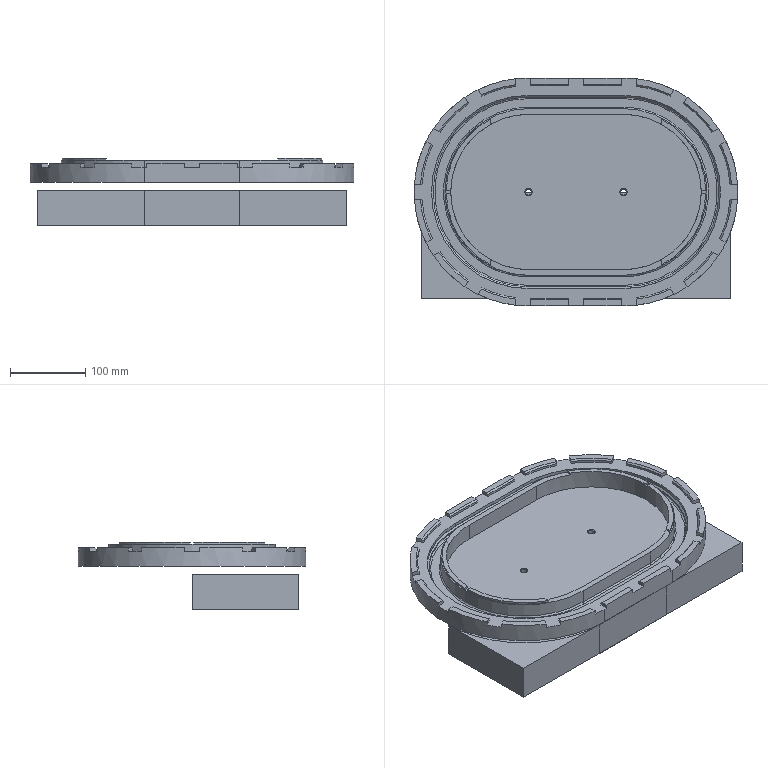NC program | NX | posted with a generic post | part box 429 x 302 x 89.371 mm
Lines 1 to 770 of 53366:
(FIXTURE OFFSET VALUES ARE NOT UNIQUE FOR OPERATION FLOOR_FACING  -- PLEASE FIX)
N10 G17 G21 G94 G90
(ADAPTIVE_MILLING , TOOL : D16开粗)
N12 T02 M6
N14 G53
N16 G17 G0 G90 X-232.529 Y-1.415 S6500 M3
N18 G43 Z20. H2
N20 Z-31.
N22 G94 G1 X-232.379 Y-1.406 Z-31.937 F3000.
N24 X-232.23 Y-1.398 Z-32.308
N26 X-232.08 Y-1.389 Z-32.58
N28 X-231.93 Y-1.381 Z-32.8
N30 X-231.78 Y-1.372 Z-32.984
N32 X-231.631 Y-1.364 Z-33.142
N34 X-231.481 Y-1.355 Z-33.28
N36 X-231.331 Y-1.347 Z-33.4
N38 X-231.181 Y-1.338 Z-33.505
N40 X-231.032 Y-1.33 Z-33.598
N42 X-230.882 Y-1.321 Z-33.679
N44 X-230.732 Y-1.313 Z-33.75
N46 X-230.582 Y-1.304 Z-33.81
N48 X-230.433 Y-1.296 Z-33.862
N50 X-230.283 Y-1.287 Z-33.905
N52 X-230.133 Y-1.279 Z-33.939
N54 X-229.983 Y-1.27 Z-33.966
N56 X-229.834 Y-1.262 Z-33.985
N58 X-229.684 Y-1.253 Z-33.996
N60 X-229.534 Y-1.245 Z-34.
N62 X-226.917 Y-1.096
N64 G3 X-225.549 Y-0.177 R1.617
N66 X-224.627 Y3.205 R11.466
N68 X-224.105 Y11.109 R67.695
N70 X-224.002 Y29.525 R929.478
N72 G1 X-224.001 Y149.336
N74 G2 X-222.03 Y154.597 R8.092
N76 X-216.722 Y158.309 R13.128
N78 X-209.837 Y159.921 R26.791
N80 X-200.067 Y160.43 R100.439
N82 X-184.767 Y160.499 R886.028
N84 G1 X212.96 Y160.5
N86 G2 X218.194 Y158.455 R8.149
N88 X221.849 Y153.13 R13.214
N90 X223.433 Y146.242 R27.174
N92 X223.93 Y136.584 R101.793
N94 X223.998 Y121.509 R876.287
N96 G1 X224. Y-149.447
N98 G2 X221.953 Y-154.681 R8.155
N100 X216.79 Y-158.27 R13.129
N102 X209.801 Y-159.912 R26.786
N104 X200.368 Y-160.412 R98.806
N106 X185.181 Y-160.485 R867.12
N108 G1 X-212.947 Y-160.499
N110 G2 X-218.096 Y-158.53 R8.104
N112 X-221.786 Y-153.276 R13.109
N114 X-223.426 Y-146.287 R26.807
N116 X-223.929 Y-136.629 R100.476
N118 X-223.998 Y-121.555 R873.122
N120 G1 X-223.999 Y-6.092
N122 G2 X-223.592 Y-0.936 R45.524
N124 G3 X-223.011 Y4.707 R170.373
N126 G1 X-222.988 Y5.977
N128 G3 X-222.621 Y13.006 R221.819
N130 X-222.505 Y32.116 R969.659
N132 G1 X-222.501 Y39.761
N134 X-222.498 Y145.061
N136 G2 X-218.605 Y153.385 R11.548
N138 X-212.066 Y157.02 R17.533
N140 X-204.007 Y158.511 R37.333
N142 X-192.881 Y158.949 R147.59
N144 X-178.031 Y158.998 R940.15
N146 G1 X-77.125 Y158.999
N148 X-75.717 Y159.132
N150 X-69.613 Y159.483
N152 X-63.5 Y159.6
N154 X63.5
N156 X69.485 Y159.488
N158 G3 X77.206 Y159.103 R215.643
N160 X93.38 Y159.005 R838.433
N162 G1 X103.274 Y159.
N164 X208.573 Y158.996
N166 G2 X216.893 Y155.099 R11.533
N168 X220.497 Y148.642 R17.473
N170 X222.005 Y140.586 R36.848
N172 X222.455 Y128.786 R152.827
N174 G1 X222.498 Y115.173
N176 X222.499 Y13.629
N178 X222.631 Y12.223
N180 X222.983 Y6.118
N182 X223.1 Y0.005
N184 X222.983 Y-6.108
N186 G3 X222.61 Y-13.03 R293.259
N188 X222.504 Y-29.867 R840.804
N190 G1 X222.5 Y-37.287
N192 Y-144.836
N194 G2 X218.756 Y-153.229 R11.495
N196 X212.224 Y-156.955 R17.308
N198 X204.172 Y-158.483 R36.616
N200 X192.484 Y-158.94 R149.137
N202 X178.872 Y-158.985 R897.131
N204 G1 X77.226 Y-158.989
N206 X75.717 Y-159.132
N208 X69.613 Y-159.483
N210 X63.5 Y-159.6
N212 X-63.5
N214 X-69.485 Y-159.488
N216 G3 X-77.634 Y-159.092 R207.139
N218 X-95.274 Y-158.996 R929.441
N220 G1 X-208.336 Y-159.
N222 G2 X-216.884 Y-155.102 R11.537
N224 X-220.524 Y-148.547 R17.523
N226 X-222.012 Y-140.487 R37.347
N228 X-222.455 Y-128.798 R153.736
N230 G1 X-222.497 Y-115.186
N232 X-222.499 Y-13.648
N234 X-222.618 Y-12.392
N236 X-222.977 Y-6.275
N238 X-223.1 Y-0.15
N240 X-222.988 Y5.977
N242 X-222.641 Y12.094
N244 X-222.06 Y18.194
N246 X-221.379 Y23.365
N248 G3 X-221.041 Y33.74 R150.871
N250 G1 X-221.003 Y46.401
N252 X-221.002 Y140.561
N254 G2 X-219.826 Y146.816 R14.804
N256 X-214.016 Y153.235 R14.585
N258 X-206.467 Y156.113 R23.96
N260 X-196.979 Y157.221 R59.53
N262 X-181.908 Y157.487 R337.478
N264 G1 X-174.258 Y157.497
N266 X-89.329 Y157.498
N268 G3 X-87.862 Y157.73 R13.362
N270 G1 X-81.802 Y158.547
N272 X-76.987 Y159.01
N274 X-81.802 Y158.547
N276 X-87.862 Y157.73
N278 G2 X-92.626 Y156.952 R81.131
N280 X-100.369 Y156.639 R93.258
N282 G1 X-112.778 Y156.599
N284 X-174.266 Y156.597
N286 G3 X-193.614 Y156.428 R682.499
N288 X-203.585 Y155.591 R77.967
N290 X-210.899 Y153.436 R27.183
N292 X-217.003 Y148.242 R14.556
N294 X-219.311 Y142.035 R17.243
N296 X-219.99 Y134.422 R50.706
N298 X-220.102 Y117.548 R684.834
N300 G1 X-220.103 Y47.253
N302 G2 X-220.211 Y30.219 R872.426
N304 G1 X-221.244 Y24.267
N306 X-221.409 Y23.04
N308 X-221.244 Y24.267
N310 X-220.197 Y30.304
N312 G3 X-219.238 Y34.912 R118.578
N314 X-218.707 Y43.058 R70.838
N316 X-218.602 Y62.936 R967.012
N318 G1 X-218.601 Y119.273
N320 G2 X-218.463 Y133.672 R440.696
N322 X-217.731 Y140.6 R40.905
N324 X-210.721 Y150.549 R15.216
N326 X-203.011 Y153.582 R24.515
N328 X-193.421 Y154.775 R58.816
N330 X-178.351 Y155.082 R304.745
N332 G1 X-170.251 Y155.096
N334 X-114.418 Y155.098
N336 G3 X-100.896 Y155.158 R824.714
N338 G2 X-93.885 Y156.681 R503.045
N340 G1 X-91.557 Y157.086
N342 X-93.885 Y156.681
N344 X-99.864 Y155.402
N346 G2 X-103.132 Y154.666 R28.054
N348 X-109.994 Y154.271 R63.977
N350 X-124.591 Y154.198 R822.936
N352 G1 X-169.541 Y154.196
N354 G3 X-189.339 Y154.02 R694.539
N356 X-199.536 Y153.182 R83.166
N358 X-207.296 Y150.944 R28.996
N360 X-215.784 Y141.611 R15.806
N362 X-217.281 Y134.243 R30.094
N364 X-217.672 Y123.791 R127.733
N366 G1 X-217.702 Y110.966
N368 X-217.703 Y58.729
N370 G2 X-217.881 Y41.554 R516.659
N372 G1 X-217.963 Y40.058
N374 G3 X-219.317 Y34.426 R101.735
N376 G2 X-217.963 Y40.058 R101.735
N378 G3 X-217.086 Y43.448 R419.213
N380 X-216.413 Y49.955 R43.811
N382 X-216.207 Y64.518 R365.227
N384 G1 X-216.202 Y72.836
N386 X-216.199 Y114.524
N388 G2 X-216.023 Y129.146 R383.662
N390 X-215.134 Y136.961 R45.597
N392 X-211.69 Y144.344 R17.332
N394 X-204.611 Y149.501 R18.475
N396 X-196.373 Y151.708 R33.165
N398 X-185.273 Y152.54 R95.162
N400 X-163.562 Y152.697 R888.938
N402 G1 X-125.668 Y152.698
N404 G3 X-109.55 Y152.821 R598.221
N406 G1 X-109.313 Y152.854
N408 G2 X-101.864 Y154.893 R118.972
N410 G3 X-110.176 Y152.599 R133.755
N412 G2 X-115.078 Y151.998 R26.106
N414 X-128.084 Y151.801 R294.067
N416 G1 X-133.028 Y151.798
N418 X-165.041 Y151.796
N420 G3 X-185.177 Y151.621 R728.917
N422 X-195.823 Y150.767 R88.315
N424 X-203.814 Y148.524 R30.934
N426 X-213.134 Y138.522 R17.107
N428 X-214.778 Y130.957 R31.176
N430 X-215.254 Y120.621 R113.28
N432 X-215.301 Y106.109 R907.702
N434 G1 X-215.303 Y68.742
N436 G2 X-215.474 Y51.781 R519.848
N438 X-215.711 Y47.993 R58.537
N440 G1 X-217.207 Y42.922
N442 G2 X-214.923 Y50.388 R168.049
N444 G3 X-214.122 Y56.177 R32.13
N446 X-213.83 Y67.138 R197.125
N448 G1 X-213.802 Y80.374
N450 X-213.8 Y109.124
N452 G2 X-213.632 Y124.422 R448.239
N454 X-212.785 Y132.808 R55.119
N456 X-210.096 Y139.93 R20.672
N458 X-202.625 Y146.474 R18.231
N460 X-194.156 Y149.085 R31.148
N462 X-183.409 Y150.071 R81.805
N464 X-164.174 Y150.293 R571.096
N466 G1 X-157.311 Y150.297
N468 X-131.858 Y150.299
N470 G3 X-117.275 Y150.464 R399.813
N472 X-116.456 Y150.541 R5.706
N474 G1 X-111.653 Y152.163
N476 X-110.142 Y152.609
N478 X-111.653 Y152.163
N480 G2 X-117.413 Y150.235 R545.021
N482 X-122.514 Y149.607 R26.689
N484 X-134.835 Y149.402 R272.839
N486 G1 X-139.778 Y149.398
N488 X-160.428 Y149.396
N490 G3 X-181.127 Y149.225 R789.564
N492 X-192.114 Y148.387 R95.379
N494 X-200.459 Y146.139 R33.132
N496 X-210.577 Y135.496 R18.152
N498 X-212.338 Y127.494 R32.811
N500 X-212.843 Y117.16 R113.078
N502 X-212.902 Y100.623 R967.326
N504 G1 X-212.904 Y76.729
N506 G2 X-213.087 Y59.665 R500.906
N508 X-213.44 Y54.677 R64.548
N510 G3 X-215.012 Y50.08 R526.691
N512 G2 X-212.748 Y56.461 R110.245
N514 G3 X-211.846 Y61.666 R25.257
N516 X-211.457 Y71.559 R135.437
N518 X-211.402 Y87.236 R942.517
N520 G1 X-211.4 Y104.399
N522 G2 X-211.242 Y120.147 R508.259
N524 X-210.384 Y129.211 R62.267
N526 X-207.781 Y136.604 R22.953
N528 X-199.911 Y143.847 R18.735
N530 X-191.359 Y146.58 R31.313
N532 X-180.73 Y147.632 R78.833
N534 X-163.183 Y147.888 R458.463
N536 G1 X-152.721 Y147.897
N538 X-138.834 Y147.899
N540 G3 X-124.489 Y148.081 R360.078
N542 X-122.708 Y148.211 R16.953
N544 G2 X-117.019 Y150.351 R524.72
N546 G3 X-123.159 Y148.03 R553.774
N548 G2 X-127.343 Y147.323 R18.935
N550 X-137.456 Y147.019 R146.156
N552 G1 X-145.741 Y146.998
N554 X-156.716 Y146.996
N556 G3 X-177.302 Y146.83 R821.488
N558 X-188.517 Y146.014 R102.546
N560 X-197.208 Y143.771 R35.317
N562 X-205.569 Y137.284 R19.163
N564 X-209.058 Y129.285 R22.631
N566 X-210.227 Y120.259 R51.32
N568 X-210.493 Y105.863 R292.52
N570 G1 X-210.502 Y98.213
N572 X-210.504 Y83.817
N574 G2 X-210.697 Y66.536 R493.875
N576 X-211.165 Y60.586 R65.041
N578 X-211.536 Y59.644 R8.23
N580 G1 X-212.777 Y56.384
N582 G2 X-210.523 Y62.026 R88.882
N584 G3 X-209.526 Y67.119 R22.594
N586 X-209.067 Y77.308 R121.258
N588 X-209.004 Y90.5 R803.915
N590 G1 X-208.996 Y103.412
N592 G2 X-208.764 Y118.259 R341.857
N594 X-207.712 Y127.186 R53.849
N596 X-204.575 Y134.855 R22.208
N598 X-196.507 Y141.622 R19.769
N600 X-187.686 Y144.256 R33.605
N602 X-176.826 Y145.25 R86.624
N604 X-158.154 Y145.49 R531.312
N606 G1 X-147.27 Y145.497
N608 G3 X-131.761 Y145.647 R487.614
N610 X-128.321 Y145.871 R68.566
N612 G1 X-128.099 Y145.928
N614 X-123.159 Y148.03
N616 G2 X-128.816 Y145.645 R224.786
N618 X-132.979 Y144.939 R20.115
N620 X-143.308 Y144.62 R146.421
N622 G1 X-155.395 Y144.593
N624 G3 X-175.194 Y144.386 R644.825
N626 X-186.175 Y143.477 R93.764
N628 X-194.823 Y141.082 R34.447
N630 X-203.82 Y133.328 R19.496
N632 X-206.84 Y125.249 R25.301
N634 X-207.877 Y115.753 R61.175
N636 X-208.095 Y101.243 R367.634
N638 G1 X-208.105 Y90.005
N640 G2 X-208.295 Y72.943 R496.233
N642 X-208.899 Y65.865 R61.317
N644 X-209.138 Y65.282 R4.531
N646 G1 X-210.547 Y61.969
N648 G2 X-208.252 Y67.195 R119.991
N650 G3 X-207.2 Y72.151 R21.284
N652 X-206.692 Y81.725 R106.769
N654 X-206.599 Y98.156 R894.507
N656 G2 X-206.385 Y114.354 R417.318
N658 X-205.414 Y123.519 R61.188
N660 X-202.505 Y131.405 R24.313
N662 X-193.932 Y139.04 R20.065
N664 X-185.143 Y141.753 R33.55
N666 X-173.953 Y142.831 R84.518
N668 X-157.194 Y143.084 R458.578
N670 G1 X-145.952 Y143.111
N672 G3 X-134.898 Y143.397 R173.963
N674 X-133.171 Y143.587 R13.575
N676 X-128.474 Y145.769 R267.332
N678 G1 X-133.444 Y143.44
N680 G2 X-137.038 Y142.67 R14.728
N682 X-145.071 Y142.263 R87.833
N684 X-160.048 Y142.172 R967.726
N686 G3 X-175.904 Y141.797 R299.023
N688 X-186.271 Y140.47 R65.391
N690 X-194.54 Y137.316 R28.173
N692 X-203.021 Y127.106 R19.971
N694 X-204.989 Y118.69 R34.917
N696 X-205.61 Y108.025 R106.855
N698 X-205.711 Y91.485 R913.213
N700 G2 X-205.992 Y76.759 R299.721
N702 X-206.668 Y70.553 R45.214
N704 G1 X-208.383 Y66.884
N706 G2 X-206.008 Y71.86 R296.464
N708 G3 X-204.919 Y76.452 R19.24
N710 X-204.319 Y85.92 R89.818
N712 X-204.175 Y102.001 R941.513
N714 G2 X-203.754 Y114.816 R181.419
N716 X-202.312 Y123.342 R42.863
N718 X-197.578 Y131.934 R21.081
N720 X-189.315 Y137.394 R22.316
N722 X-179.94 Y139.69 R40.337
N724 X-167.712 Y140.532 R115.893
N726 X-150.024 Y140.714 R917.51
N728 G3 X-139.469 Y141.06 R145.435
N730 X-137.692 Y141.292 R10.352
N732 G1 X-134.315 Y143.029
N734 X-133.399 Y143.461
N736 G3 X-137.877 Y141.18 R113.782
N738 G2 X-141.24 Y140.36 R12.781
N740 X-149.269 Y139.876 R77.466
N742 X-162.445 Y139.724 R997.313
N744 G3 X-176.266 Y139.128 R177.234
N746 X-185.993 Y137.362 R49.79
N748 X-194.278 Y133.151 R24.354
N750 X-200.723 Y123.933 R20.835
N752 X-202.616 Y115.386 R37.202
N754 X-203.224 Y104.156 R118.396
N756 X-203.338 Y91.539 R848.814
N758 G2 X-203.751 Y79.751 R171.159
N760 X-204.436 Y74.878 R34.133
N762 G1 X-206.136 Y71.572
N764 X-203.715 Y76.265
N766 G3 X-202.562 Y80.981 R19.372
N768 X-201.946 Y89.782 R82.903
N770 X-201.736 Y102.722 R902.7
N772 G2 X-201.138 Y113.952 R121.489
N774 X-199.225 Y122.495 R35.576
N776 X-189.076 Y133.824 R20.616
N778 X-180.128 Y136.775 R33.287
N780 X-169.063 Y137.966 R79.662
N782 X-155.447 Y138.285 R378.224
N784 G3 X-144.611 Y138.641 R167.502
N786 X-142.021 Y138.957 R20.136
N788 G1 X-141.794 Y139.044
N790 G2 X-137.844 Y141.197 R66.863
N792 G3 X-142.088 Y138.877 R70.749
N794 G2 X-145.474 Y138.006 R12.512
N796 X-153.148 Y137.476 R71.347
N798 G1 X-164.09 Y137.234
N800 G3 X-176.317 Y136.379 R117.575
N802 X-185.689 Y134.075 R39.995
N804 X-194.12 Y128.323 R21.894
N806 X-198.764 Y119.769 R22.771
N808 X-200.389 Y110.705 R44.506
N810 X-200.873 Y99.13 R167.521
N812 G2 X-201.233 Y86.251 R299.634
N814 X-202.123 Y79.17 R45.234
N816 G1 X-202.246 Y78.819
N818 X-203.811 Y76.05
N820 X-201.482 Y80.193
N822 G3 X-200.258 Y84.8 R18.25
N824 X-199.559 Y93.549 R80.328
N826 G2 X-199.157 Y105.736 R888.13
N828 X-198.059 Y115.339 R63.526
N830 X-194.989 Y123.52 R26.02
N832 X-186.036 Y131.565 R21.185
N834 X-176.934 Y134.434 R34.78
N836 X-165.975 Y135.574 R84.23
N838 X-153.798 Y135.971 R849.201
N840 G3 X-146.27 Y136.57 R64.398
N842 X-145.763 Y136.75 R4.13
N844 G2 X-142.024 Y138.914 R85.291
N846 G3 X-146.05 Y136.572 R95.169
N848 G2 X-149.311 Y135.66 R11.602
N850 X-156.846 Y135.036 R68.442
N852 G3 X-168.491 Y134.485 R359.878
N854 X-178.721 Y132.991 R62.429
N856 X-187.217 Y129.504 R28.342
N858 X-195.619 Y119.119 R21.192
N860 X-197.729 Y110.276 R36.881
N862 X-198.455 Y99.505 R121.199
N864 G2 X-199.004 Y88.472 R198.973
N866 X-199.881 Y82.931 R35.355
N868 G1 X-199.982 Y82.695
N870 G3 X-201.63 Y79.902 R56.352
N872 G2 X-199.389 Y83.651 R71.76
N874 G3 X-198.103 Y87.599 R14.334
N876 X-197.23 Y95.299 R59.584
N878 G2 X-196.596 Y105.782 R494.055
N880 X-195.152 Y114.653 R49.361
N882 X-190.883 Y123.269 R23.267
N884 X-182.366 Y129.607 R22.421
N886 X-173.186 Y132.197 R38.111
N888 X-162.553 Y133.236 R99.8
N890 G3 X-153.14 Y133.81 R258.501
N892 X-149.863 Y134.27 R33.895
N894 G1 X-149.551 Y134.399
N896 X-146.014 Y136.594
N898 X-149.838 Y134.221
N900 G2 X-152.962 Y133.282 R11.534
N902 X-159.312 Y132.579 R62.01
N904 G3 X-169.26 Y131.76 R217.506
N906 X-178.931 Y129.727 R47.487
N908 X-187.326 Y125.027 R24.367
N910 X-193.497 Y115.66 R22.216
N912 X-195.415 Y107. R40.564
N914 X-196.199 Y97.313 R169.715
N916 G2 X-197.097 Y88.799 R77.617
N918 X-197.634 Y86.505 R18.479
N920 G1 X-199.409 Y83.618
N922 X-197.031 Y87.422
N924 G3 X-195.672 Y91.568 R15.382
N926 X-194.767 Y98.229 R66.194
N928 G2 X-193.781 Y107.15 R159.087
N930 X-191.492 Y115.603 R34.646
N932 X-181.082 Y126.549 R21.644
N934 X-171.899 Y129.546 R35.313
N936 X-162.868 Y130.732 R90.72
N938 G3 X-155.159 Y131.552 R127.176
N940 X-153.358 Y131.913 R13.814
N942 G1 X-153.124 Y132.025
N944 G2 X-149.772 Y134.261 R152.245
N946 G3 X-153.404 Y131.836 R162.206
N948 G2 X-156.364 Y130.842 R11.194
N950 X-162.337 Y129.946 R65.092
N952 G3 X-171.462 Y128.612 R104.727
N954 X-180.279 Y125.63 R34.085
N956 X-190.699 Y114.087 R21.884
N958 X-192.935 Y105.501 R38.719
N960 X-194.031 Y96.683 R281.796
N962 G2 X-195.27 Y90.134 R40.815
N964 G1 X-195.435 Y89.757
N966 X-197.197 Y87.147
N968 G3 X-194.621 Y90.996 R147.309
N970 X-193.131 Y95.401 R17.491
N972 X-191.826 Y102.887 R141.538
N974 G2 X-189.876 Y111.086 R48.243
N976 X-183.95 Y120.383 R22.723
N978 X-175.286 Y125.52 R25.341
N980 X-166.121 Y127.772 R50.643
N982 G3 X-158.637 Y128.978 R282.809
N984 X-156.942 Y129.391 R10.268
N986 G1 X-156.745 Y129.499
N988 G2 X-153.359 Y131.866 R63.417
N990 G3 X-157.017 Y129.299 R66.548
N992 G2 X-160.043 Y128.163 R11.885
N994 X-166.732 Y126.768 R133.646
N996 G3 X-175.273 Y124.351 R47.644
N998 X-183.883 Y118.583 R23.72
N1000 X-188.97 Y109.888 R24.411
N1002 X-190.989 Y101.819 R55.382
N1004 G2 X-192.449 Y94.84 R91.224
N1006 X-192.949 Y93.327 R9.609
N1008 G3 X-194.793 Y90.707 R70.089
N1010 G2 X-192.275 Y94.233 R81.048
N1012 G3 X-190.655 Y98.1 R16.248
N1014 X-188.866 Y104.735 R322.928
N1016 G2 X-185.871 Y112.374 R34.392
N1018 X-175.833 Y121.824 R23.043
N1020 X-167.581 Y124.777 R41.314
N1022 G3 X-161.416 Y126.325 R379.706
N1024 X-160.25 Y126.931 R2.341
N1026 G1 X-156.983 Y129.324
N1028 G3 X-160.86 Y126.448 R130.955
N1030 G2 X-163.791 Y125.124 R13.101
N1032 G1 X-169.878 Y123.158
N1034 G3 X-177.662 Y119.409 R32.564
N1036 X-185.861 Y109.566 R23.743
N1038 X-188.386 Y102.579 R50.642
N1040 G2 X-190.092 Y97.248 R73.13
N1042 X-190.425 Y96.758 R3.493
N1044 G1 X-192.286 Y94.217
N1046 G2 X-189.397 Y98.055 R72.895
N1048 G3 X-187.482 Y101.798 R21.048
N1050 G2 X-184.801 Y107.935 R97.855
N1052 X-176.996 Y117.321 R25.289
N1054 X-169.357 Y121.384 R35.147
N1056 G1 X-165.354 Y122.931
N1058 X-165.041 Y123.133
N1060 X-160.81 Y126.488
N1062 X-165.677 Y122.617
N1064 G2 X-168.65 Y120.939 R26.85
N1066 G3 X-174.528 Y117.682 R58.062
N1068 X-183.554 Y107.751 R27.028
N1070 X-186.48 Y101.769 R113.604
N1072 G1 X-186.626 Y101.549
N1074 X-189.422 Y98.023
N1076 G2 X-184.803 Y103.688 R132.321
N1078 G3 X-181.624 Y108.167 R498.29
N1080 G2 X-171.953 Y117.078 R33.192
N1082 G3 X-169.682 Y119.153 R55.725
N1084 G1 X-165.412 Y122.814
N1086 X-169.682 Y119.153
N1088 X-174.168 Y114.999
N1090 X-178.492 Y110.676
N1092 X-182.646 Y106.19
N1094 X-184.916 Y103.543
N1096 G2 X-186.671 Y103.077 R1.603
N1098 G1 X-189.668 Y104.035 Z-33.9
N1100 X-190.008 Y104.146 F15000.
N1102 X-190.352 Y104.242
N1104 G3 X-191.997 Y103.543 R1.6
N1106 G1 X-201.643 Y88.697
N1108 G3 X-209.964 Y74.237 R156.698
N1110 X-219.209 Y52.045 R153.871
N1112 X-222.647 Y40.259 R185.878
N1114 X-226.149 Y22.272 R159.931
N1116 X-227.008 Y14.46 R192.013
N1118 X-227.982 Y1.392 R369.431
N1120 G1 X-228.631 Y-10.074
N1122 G3 X-227.238 Y-11.752 R1.6
N1124 G1 X-226.609 Y-11.833
N1126 X-225.182 Y-12.013 Z-33.946 F3000.
N1128 X-223.755 Y-12.205 Z-33.991
N1130 X-223.499 Y-12.284 Z-34.
N1132 G2 X-222.499 Y-13.615 R1.6
N1134 X-221.814 Y-20.81 R304.339
N1136 X-221.608 Y-32.307 R229.116
N1138 G1 X-221.599 Y-41.066
N1140 X-221.597 Y-115.829
N1142 G3 X-221.431 Y-134.165 R623.958
N1144 X-220.634 Y-143.348 R69.881
N1146 X-218.547 Y-150.098 R23.675
N1148 X-211.468 Y-156.376 R12.438
N1150 X-204.764 Y-157.746 R25.7
N1152 X-195.434 Y-158.073 R120.939
N1154 G1 X-183.622 Y-158.099
N1156 X-93.994 Y-158.097
N1158 X-84.972 Y-158.122
N1160 X-81.421 Y-158.591
N1162 X-75.461 Y-159.151
N1164 X-81.421 Y-158.591
N1166 X-87.355 Y-157.807
N1168 G3 X-91.838 Y-157.065 R139.171
N1170 X-101.536 Y-156.65 R109.757
N1172 X-117.549 Y-156.597 R976.687
N1174 G1 X-187.136 Y-156.596
N1176 G2 X-200.409 Y-156.429 R328.503
N1178 X-207.1 Y-155.613 R35.748
N1180 X-215.62 Y-149.538 R13.905
N1182 X-218.598 Y-142.279 R22.394
N1184 X-219.774 Y-133.254 R53.604
N1186 X-220.083 Y-118.634 R283.141
N1188 G1 X-220.097 Y-109.297
N1190 X-220.098 Y-44.279
N1192 G3 X-220.136 Y-30.613 R896.441
N1194 G1 X-221.199 Y-24.562
N1196 X-221.988 Y-18.765
N1198 X-221.199 Y-24.562
N1200 X-220.136 Y-30.613
N1202 G2 X-219.367 Y-36.566 R28.313
N1204 X-219.205 Y-48.39 R315.265
N1206 G1 X-219.199 Y-55.803
N1208 X-219.197 Y-109.866
N1210 G3 X-219.037 Y-128.764 R695.637
N1212 X-218.22 Y-138.736 R78.589
N1214 X-216.06 Y-146.049 R26.602
N1216 X-207.799 Y-153.619 R14.776
N1218 X-200.461 Y-155.239 R28.04
N1220 X-190.461 Y-155.661 R112.868
N1222 G1 X-177.524 Y-155.699
N1224 X-114.354
N1226 G2 X-97.8 Y-155.853 R561.178
N1228 G1 X-93.256 Y-156.802
N1230 X-91.37 Y-157.123
N1232 G2 X-97.775 Y-155.856 R123.101
N1234 X-101.588 Y-154.971 R83.467
N1236 G3 X-108.769 Y-154.355 R52.906
N1238 X-125.651 Y-154.199 R560.051
N1240 G1 X-175.236
N1242 G2 X-193.21 Y-154.085 R755.921
N1244 X-201.387 Y-153.4 R58.826
N1246 X-207.646 Y-151.294 R19.204
N1248 X-213.883 Y-144.687 R16.178
N1250 X-216.447 Y-137.007 R27.162
N1252 X-217.46 Y-127.054 R69.261
N1254 X-217.69 Y-110.857 R429.837
N1256 G1 X-217.698 Y-100.057
N1258 X-217.701 Y-52.048
N1260 G3 X-217.786 Y-40.811 R697.321
N1262 X-218.85 Y-36.587 R190.96
N1264 G1 X-219.797 Y-32.188
N1266 G3 X-217.804 Y-40.675 R133.401
N1268 G2 X-217.025 Y-45.791 R22.201
N1270 X-216.809 Y-56.386 R211.425
N1272 G1 X-216.798 Y-64.466
N1274 X-216.796 Y-104.691
N1276 G3 X-216.627 Y-124.489 R715.462
N1278 X-215.784 Y-134.798 R82.881
N1280 X-213.532 Y-142.556 R28.702
N1282 X-204.379 Y-151.036 R16.337
N1284 X-196.72 Y-152.767 R29.917
N1286 X-186.61 Y-153.248 R108.619
N1288 X-171.31 Y-153.298 R931.317
N1290 G1 X-126.279
N1292 G2 X-109.317 Y-153.468 R529.07
N1294 X-106.681 Y-153.623 R35.142
N1296 G3 X-101.321 Y-155.027 R100.077
N1298 G2 X-109.491 Y-152.811 R137.348
N1300 G3 X-115.352 Y-152.077 R35.4
N1302 X-128.478 Y-151.81 R259.983
N1304 G1 X-139.261 Y-151.798
N1306 X-175.099 Y-151.796
N1308 G2 X-190.509 Y-151.614 R411.776
N1310 X-198.776 Y-150.713 R50.837
N1312 X-205.814 Y-147.843 R19.303
N1314 X-211.674 Y-140.825 R17.766
N1316 X-214.128 Y-132.771 R30.284
N1318 X-215.085 Y-122.247 R79.668
N1320 X-215.292 Y-104.924 R529.268
N1322 G1 X-215.298 Y-95.587
N1324 X-215.299 Y-63.184
N1326 G3 X-215.45 Y-48.905 R404.662
N1328 X-215.585 Y-48.396 R4.353
N1330 G2 X-217.498 Y-41.869 R232.953
N1332 G3 X-215.198 Y-49.588 R202.063
N1334 G2 X-214.606 Y-54.403 R26.507
N1336 X-214.401 Y-67.397 R283.072
N1338 G1 X-214.398 Y-72.341
N1340 X-214.396 Y-100.303
N1342 G3 X-214.233 Y-120.102 R761.481
N1344 X-213.405 Y-130.864 R91.575
N1346 X-211.179 Y-138.976 R31.496
N1348 X-201.01 Y-148.57 R17.559
N1350 X-193.126 Y-150.33 R32.018
N1352 X-183.018 Y-150.837 R109.295
N1354 X-167.718 Y-150.898 R896.73
N1356 G1 X-135.391 Y-150.899
N1358 G2 X-118.324 Y-151.077 R514.395
N1360 X-114.001 Y-151.371 R44.635
N1362 G3 X-109.485 Y-152.813 R97.147
N1364 G2 X-114.001 Y-151.371 R97.147
N1366 G3 X-117.025 Y-150.422 R38.254
N1368 X-123.315 Y-149.668 R39.048
N1370 X-138.146 Y-149.405 R320.002
N1372 G1 X-146.461 Y-149.398
N1374 X-170.261 Y-149.396
N1376 G2 X-185.897 Y-149.234 R487.426
N1378 X-194.736 Y-148.384 R60.418
N1380 X-202.107 Y-145.733 R22.141
N1382 X-209.074 Y-137.949 R18.344
N1384 X-211.661 Y-129.594 R31.14
N1386 X-212.649 Y-119.299 R78.789
N1388 X-212.888 Y-102.426 R457.064
N1390 G1 X-212.897 Y-92.976
N1392 X-212.899 Y-71.171
N1394 G3 X-213.051 Y-57.019 R411.123
N1396 X-213.157 Y-55.43 R15.354
N1398 G2 X-215.279 Y-49.298 R191.25
N1400 G1 X-213.616 Y-54.198
N1402 G2 X-212.822 Y-56.403 R20.928
N1404 X-212.212 Y-61.382 R28.002
N1406 X-212.002 Y-73.7 R267.247
N1408 G1 X-211.998 Y-78.641
N1410 X-211.996 Y-95.916
N1412 G3 X-211.827 Y-116.39 R784.557
N1414 X-210.993 Y-127.377 R96.027
N1416 X-208.722 Y-135.827 R33.431
N1418 X-197.887 Y-146.096 R18.499
N1420 X-189.782 Y-147.899 R33.534
N1422 X-178.775 Y-148.44 R116.099
N1424 X-163.475 Y-148.498 R914.647
N1426 G1 X-142.929 Y-148.5
N1428 G2 X-125.761 Y-148.694 R484.531
N1430 X-120.374 Y-149.106 R60.989
N1432 G1 X-116.358 Y-150.593
N1434 G3 X-122.503 Y-148.32 R554.363
N1436 X-128.107 Y-147.407 R27.729
N1438 X-138.422 Y-147.044 R149.956
N1440 X-153.661 Y-146.999 R963.406
N1442 G1 X-165.874 Y-146.996
N1444 G2 X-182.634 Y-146.813 R483.698
N1446 X-191.803 Y-145.885 R60.743
N1448 X-199.272 Y-143.166 R23.24
N1450 X-206.527 Y-135.116 R19.039
N1452 X-209.187 Y-126.651 R31.809
N1454 X-210.238 Y-115.911 R79.881
N1456 X-210.486 Y-99.263 R446.992
N1458 G1 X-210.496 Y-90.938
N1460 X-210.497 Y-80.393
N1462 G3 X-210.64 Y-64.42 R515.325
N1464 X-210.828 Y-61.379 R36.427
N1466 X-211.425 Y-59.921 R12.938
N1468 G1 X-212.993 Y-55.823
N1470 G3 X-210.71 Y-61.591 R113.852
N1472 G2 X-209.99 Y-65.322 R15.9
N1474 X-209.633 Y-74.656 R112.492
N1476 X-209.598 Y-88.855 R933.097
N1478 G1 X-209.576 Y-101.655
N1480 G3 X-209.22 Y-117.511 R302.188
N1482 X-207.942 Y-127.544 R62.893
N1484 X-204.898 Y-135.495 R26.792
N1486 X-195.304 Y-143.476 R19.037
N1488 X-187.002 Y-145.425 R33.448
N1490 X-176.673 Y-146.014 R105.087
N1492 X-161.374 Y-146.098 R845.295
N1494 G1 X-152.376 Y-146.099
N1496 G2 X-133.479 Y-146.259 R653.421
N1498 X-126.048 Y-146.835 R67.082
N1500 G1 X-125.851 Y-146.891
N1502 X-122.007 Y-148.488
N1504 X-127.745 Y-146.116
N1506 G3 X-132.964 Y-145.115 R23.623
N1508 X-144.277 Y-144.649 R136.865
N1510 X-155.914 Y-144.601 R778.278
N1512 G1 X-169.976 Y-144.576
N1514 G2 X-182.681 Y-144.216 R196.144
N1516 X-191.223 Y-142.853 R43.093
N1518 X-199.481 Y-138.423 R20.272
N1520 X-204.829 Y-130.511 R21.283
N1522 X-207.112 Y-121.36 R38.374
N1524 X-207.938 Y-109.47 R110.722
N1526 X-208.096 Y-88.434 R906.946
N1528 G3 X-208.226 Y-71.147 R633.258
N1530 X-208.494 Y-66.772 R67.107
N1532 X-209.016 Y-65.554 R6.414
N1534 G1 X-210.741 Y-61.52
N1536 G3 X-208.398 Y-66.859 R115.372